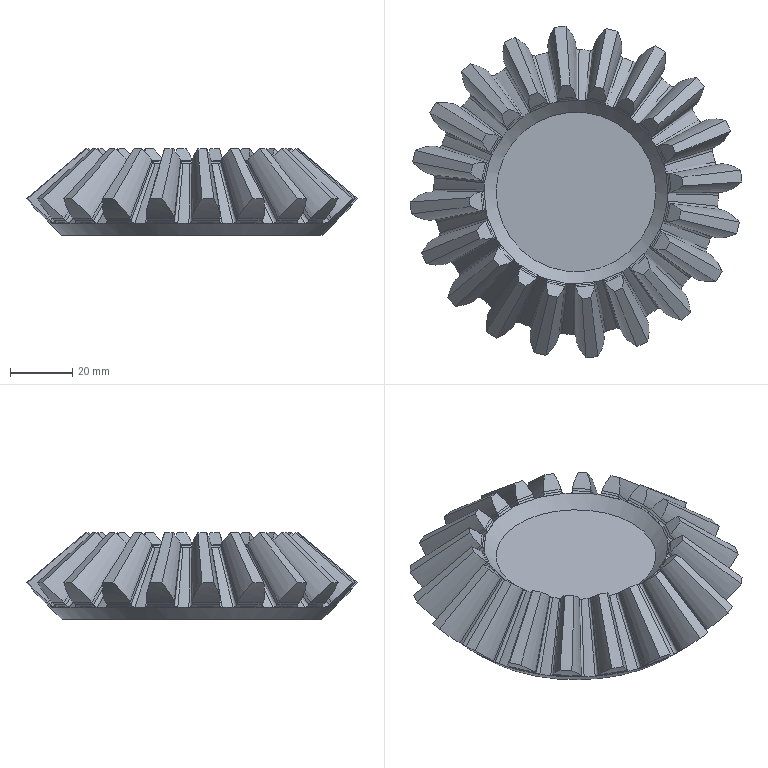Part | NX | features BREP 1 | 1 solid | 324 faces | box 106.608 x 106.608 x 27.845 mm | volume 129027 mm3 | spline 200 | plane 82 | cone 42